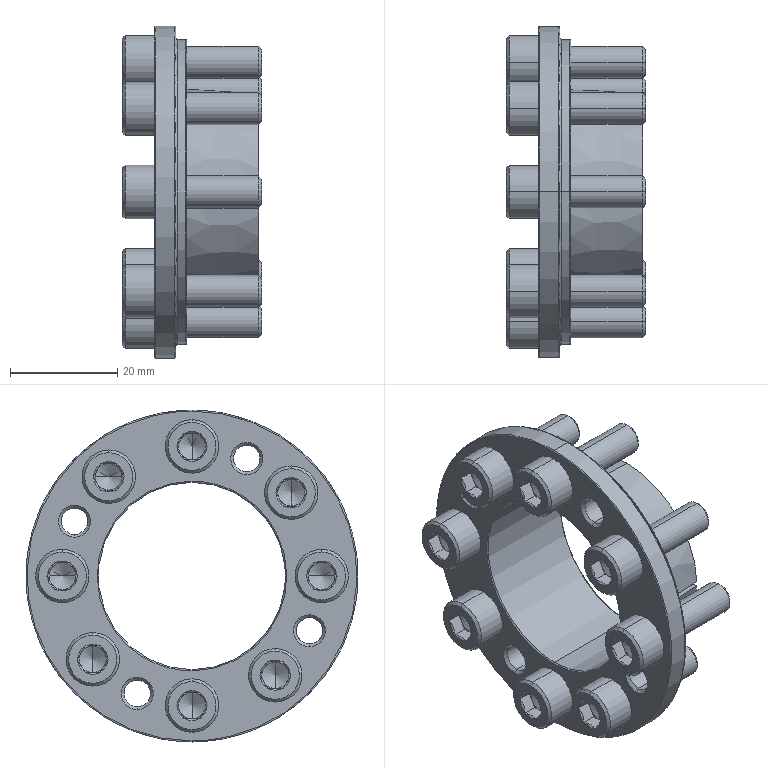Part | STEP file | expansion sleeve 35-2^PN_0025_expansion sleeve | 1 solid | 295 faces | box 26 x 62 x 62 mm | volume 19242 mm3 | cone 118 | plane 118 | cylinder 46 | spline 13 | commonest cylinder face diameters 6 x16 10 x16 4.917 x8 35 x2 57 x2 62 x2